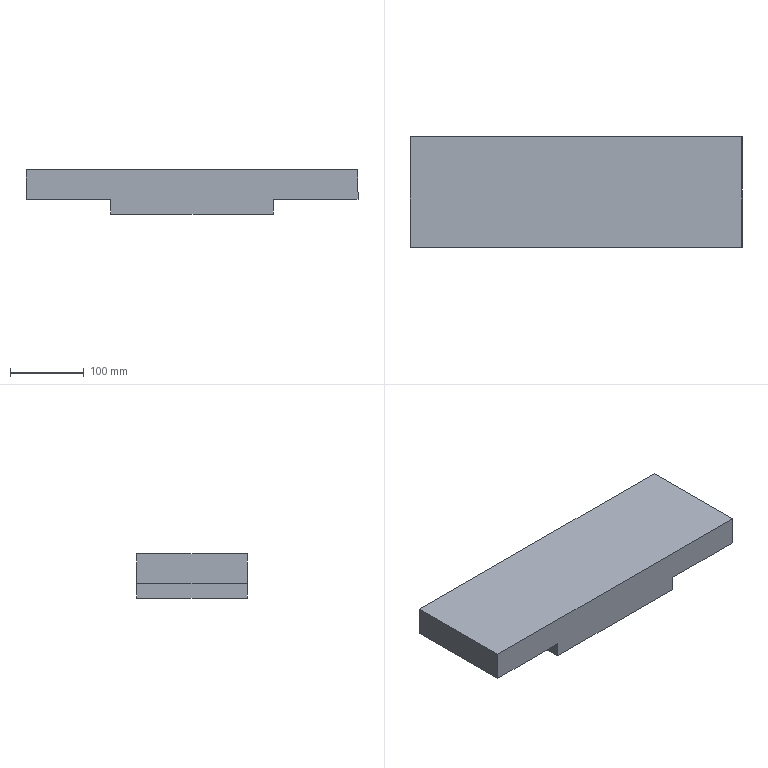Part | SolidWorks | features Extrusion 1 | 1 solid | 10 faces | box 450 x 150 x 60 mm | volume 3360000 mm3 | plane 10
STEP:
#1=CARTESIAN_POINT('',(0.,0.,0.));
#2=VERTEX_POINT('',#1);
#3=CARTESIAN_POINT('',(0.,0.,40.));
#4=VERTEX_POINT('',#3);
#5=CARTESIAN_POINT('',(0.,0.,0.));
#6=DIRECTION('',(0.,0.,1.));
#7=VECTOR('',#6,1000.);
#8=LINE('',#5,#7);
#9=EDGE_CURVE('',#2,#4,#8,.T.);
#10=ORIENTED_EDGE('',*,*,#9,.T.);
#11=CARTESIAN_POINT('',(0.,150.,40.));
#12=VERTEX_POINT('',#11);
#13=CARTESIAN_POINT('',(0.,150.,40.));
#14=DIRECTION('',(0.,-1.,0.));
#15=VECTOR('',#14,1000.);
#16=LINE('',#13,#15);
#17=EDGE_CURVE('',#12,#4,#16,.T.);
#18=ORIENTED_EDGE('',*,*,#17,.F.);
#19=CARTESIAN_POINT('',(0.,150.,0.));
#20=VERTEX_POINT('',#19);
#21=CARTESIAN_POINT('',(0.,150.,0.));
#22=DIRECTION('',(0.,0.,1.));
#23=VECTOR('',#22,1000.);
#24=LINE('',#21,#23);
#25=EDGE_CURVE('',#20,#12,#24,.T.);
#26=ORIENTED_EDGE('',*,*,#25,.F.);
#27=CARTESIAN_POINT('',(0.,150.,0.));
#28=DIRECTION('',(0.,-1.,0.));
#29=VECTOR('',#28,1000.);
#30=LINE('',#27,#29);
#31=EDGE_CURVE('',#20,#2,#30,.T.);
#32=ORIENTED_EDGE('',*,*,#31,.T.);
#33=EDGE_LOOP('',(#10,#18,#26,#32));
#34=FACE_OUTER_BOUND('',#33,.T.);
#35=CARTESIAN_POINT('',(0.,150.,0.));
#36=DIRECTION('',(1.,0.,0.));
#37=DIRECTION('',(0.,0.,-1.));
#38=AXIS2_PLACEMENT_3D('',#35,#36,#37);
#39=PLANE('',#38);
#40=ADVANCED_FACE('',(#34),#39,.F.);
#41=CARTESIAN_POINT('',(450.,0.,40.));
#42=VERTEX_POINT('',#41);
#43=CARTESIAN_POINT('',(0.,0.,40.));
#44=DIRECTION('',(1.,0.,0.));
#45=VECTOR('',#44,1000.);
#46=LINE('',#43,#45);
#47=EDGE_CURVE('',#4,#42,#46,.T.);
#48=ORIENTED_EDGE('',*,*,#47,.T.);
#49=CARTESIAN_POINT('',(450.,150.,40.));
#50=VERTEX_POINT('',#49);
#51=CARTESIAN_POINT('',(450.,150.,40.));
#52=DIRECTION('',(0.,-1.,0.));
#53=VECTOR('',#52,1000.);
#54=LINE('',#51,#53);
#55=EDGE_CURVE('',#50,#42,#54,.T.);
#56=ORIENTED_EDGE('',*,*,#55,.F.);
#57=CARTESIAN_POINT('',(0.,150.,40.));
#58=DIRECTION('',(1.,0.,0.));
#59=VECTOR('',#58,1000.);
#60=LINE('',#57,#59);
#61=EDGE_CURVE('',#12,#50,#60,.T.);
#62=ORIENTED_EDGE('',*,*,#61,.F.);
#63=ORIENTED_EDGE('',*,*,#17,.T.);
#64=EDGE_LOOP('',(#48,#56,#62,#63));
#65=FACE_OUTER_BOUND('',#64,.T.);
#66=CARTESIAN_POINT('',(0.,150.,40.));
#67=DIRECTION('',(0.,0.,-1.));
#68=DIRECTION('',(-1.,0.,0.));
#69=AXIS2_PLACEMENT_3D('',#66,#67,#68);
#70=PLANE('',#69);
#71=ADVANCED_FACE('',(#65),#70,.F.);
#72=CARTESIAN_POINT('',(450.,0.,0.));
#73=VERTEX_POINT('',#72);
#74=CARTESIAN_POINT('',(450.,0.,0.));
#75=DIRECTION('',(0.,0.,-1.));
#76=VECTOR('',#75,1000.);
#77=LINE('',#74,#76);
#78=EDGE_CURVE('',#42,#73,#77,.T.);
#79=ORIENTED_EDGE('',*,*,#78,.T.);
#80=CARTESIAN_POINT('',(450.,150.,0.));
#81=VERTEX_POINT('',#80);
#82=CARTESIAN_POINT('',(450.,150.,0.));
#83=DIRECTION('',(0.,-1.,0.));
#84=VECTOR('',#83,1000.);
#85=LINE('',#82,#84);
#86=EDGE_CURVE('',#81,#73,#85,.T.);
#87=ORIENTED_EDGE('',*,*,#86,.F.);
#88=CARTESIAN_POINT('',(450.,150.,0.));
#89=DIRECTION('',(0.,0.,-1.));
#90=VECTOR('',#89,1000.);
#91=LINE('',#88,#90);
#92=EDGE_CURVE('',#50,#81,#91,.T.);
#93=ORIENTED_EDGE('',*,*,#92,.F.);
#94=ORIENTED_EDGE('',*,*,#55,.T.);
#95=EDGE_LOOP('',(#79,#87,#93,#94));
#96=FACE_OUTER_BOUND('',#95,.T.);
#97=CARTESIAN_POINT('',(450.,150.,0.));
#98=DIRECTION('',(-1.,0.,0.));
#99=DIRECTION('',(0.,0.,1.));
#100=AXIS2_PLACEMENT_3D('',#97,#98,#99);
#101=PLANE('',#100);
#102=ADVANCED_FACE('',(#96),#101,.F.);
#103=CARTESIAN_POINT('',(335.,0.,0.));
#104=VERTEX_POINT('',#103);
#105=CARTESIAN_POINT('',(335.,0.,0.));
#106=DIRECTION('',(-1.,0.,0.));
#107=VECTOR('',#106,1000.);
#108=LINE('',#105,#107);
#109=EDGE_CURVE('',#73,#104,#108,.T.);
#110=ORIENTED_EDGE('',*,*,#109,.T.);
#111=CARTESIAN_POINT('',(335.,150.,0.));
#112=VERTEX_POINT('',#111);
#113=CARTESIAN_POINT('',(335.,150.,0.));
#114=DIRECTION('',(0.,-1.,0.));
#115=VECTOR('',#114,1000.);
#116=LINE('',#113,#115);
#117=EDGE_CURVE('',#112,#104,#116,.T.);
#118=ORIENTED_EDGE('',*,*,#117,.F.);
#119=CARTESIAN_POINT('',(335.,150.,0.));
#120=DIRECTION('',(-1.,0.,0.));
#121=VECTOR('',#120,1000.);
#122=LINE('',#119,#121);
#123=EDGE_CURVE('',#81,#112,#122,.T.);
#124=ORIENTED_EDGE('',*,*,#123,.F.);
#125=ORIENTED_EDGE('',*,*,#86,.T.);
#126=EDGE_LOOP('',(#110,#118,#124,#125));
#127=FACE_OUTER_BOUND('',#126,.T.);
#128=CARTESIAN_POINT('',(335.,150.,0.));
#129=DIRECTION('',(0.,0.,1.));
#130=DIRECTION('',(1.,0.,0.));
#131=AXIS2_PLACEMENT_3D('',#128,#129,#130);
#132=PLANE('',#131);
#133=ADVANCED_FACE('',(#127),#132,.F.);
#134=CARTESIAN_POINT('',(335.,0.,-20.));
#135=VERTEX_POINT('',#134);
#136=CARTESIAN_POINT('',(335.,0.,-20.));
#137=DIRECTION('',(0.,0.,-1.));
#138=VECTOR('',#137,1000.);
#139=LINE('',#136,#138);
#140=EDGE_CURVE('',#104,#135,#139,.T.);
#141=ORIENTED_EDGE('',*,*,#140,.T.);
#142=CARTESIAN_POINT('',(335.,150.,-20.));
#143=VERTEX_POINT('',#142);
#144=CARTESIAN_POINT('',(335.,150.,-20.));
#145=DIRECTION('',(0.,-1.,0.));
#146=VECTOR('',#145,1000.);
#147=LINE('',#144,#146);
#148=EDGE_CURVE('',#143,#135,#147,.T.);
#149=ORIENTED_EDGE('',*,*,#148,.F.);
#150=CARTESIAN_POINT('',(335.,150.,-20.));
#151=DIRECTION('',(0.,0.,-1.));
#152=VECTOR('',#151,1000.);
#153=LINE('',#150,#152);
#154=EDGE_CURVE('',#112,#143,#153,.T.);
#155=ORIENTED_EDGE('',*,*,#154,.F.);
#156=ORIENTED_EDGE('',*,*,#117,.T.);
#157=EDGE_LOOP('',(#141,#149,#155,#156));
#158=FACE_OUTER_BOUND('',#157,.T.);
#159=CARTESIAN_POINT('',(335.,150.,-20.));
#160=DIRECTION('',(-1.,0.,0.));
#161=DIRECTION('',(0.,0.,1.));
#162=AXIS2_PLACEMENT_3D('',#159,#160,#161);
#163=PLANE('',#162);
#164=ADVANCED_FACE('',(#158),#163,.F.);
#165=CARTESIAN_POINT('',(115.,0.,-20.));
#166=VERTEX_POINT('',#165);
#167=CARTESIAN_POINT('',(115.,0.,-20.));
#168=DIRECTION('',(-1.,0.,0.));
#169=VECTOR('',#168,1000.);
#170=LINE('',#167,#169);
#171=EDGE_CURVE('',#135,#166,#170,.T.);
#172=ORIENTED_EDGE('',*,*,#171,.T.);
#173=CARTESIAN_POINT('',(115.,150.,-20.));
#174=VERTEX_POINT('',#173);
#175=CARTESIAN_POINT('',(115.,150.,-20.));
#176=DIRECTION('',(0.,-1.,0.));
#177=VECTOR('',#176,1000.);
#178=LINE('',#175,#177);
#179=EDGE_CURVE('',#174,#166,#178,.T.);
#180=ORIENTED_EDGE('',*,*,#179,.F.);
#181=CARTESIAN_POINT('',(115.,150.,-20.));
#182=DIRECTION('',(-1.,0.,0.));
#183=VECTOR('',#182,1000.);
#184=LINE('',#181,#183);
#185=EDGE_CURVE('',#143,#174,#184,.T.);
#186=ORIENTED_EDGE('',*,*,#185,.F.);
#187=ORIENTED_EDGE('',*,*,#148,.T.);
#188=EDGE_LOOP('',(#172,#180,#186,#187));
#189=FACE_OUTER_BOUND('',#188,.T.);
#190=CARTESIAN_POINT('',(115.,150.,-20.));
#191=DIRECTION('',(0.,0.,1.));
#192=DIRECTION('',(1.,0.,0.));
#193=AXIS2_PLACEMENT_3D('',#190,#191,#192);
#194=PLANE('',#193);
#195=ADVANCED_FACE('',(#189),#194,.F.);
#196=CARTESIAN_POINT('',(115.,0.,0.));
#197=VERTEX_POINT('',#196);
#198=CARTESIAN_POINT('',(115.,0.,0.));
#199=DIRECTION('',(0.,0.,1.));
#200=VECTOR('',#199,1000.);
#201=LINE('',#198,#200);
#202=EDGE_CURVE('',#166,#197,#201,.T.);
#203=ORIENTED_EDGE('',*,*,#202,.T.);
#204=CARTESIAN_POINT('',(115.,150.,0.));
#205=VERTEX_POINT('',#204);
#206=CARTESIAN_POINT('',(115.,150.,0.));
#207=DIRECTION('',(0.,-1.,0.));
#208=VECTOR('',#207,1000.);
#209=LINE('',#206,#208);
#210=EDGE_CURVE('',#205,#197,#209,.T.);
#211=ORIENTED_EDGE('',*,*,#210,.F.);
#212=CARTESIAN_POINT('',(115.,150.,0.));
#213=DIRECTION('',(0.,0.,1.));
#214=VECTOR('',#213,1000.);
#215=LINE('',#212,#214);
#216=EDGE_CURVE('',#174,#205,#215,.T.);
#217=ORIENTED_EDGE('',*,*,#216,.F.);
#218=ORIENTED_EDGE('',*,*,#179,.T.);
#219=EDGE_LOOP('',(#203,#211,#217,#218));
#220=FACE_OUTER_BOUND('',#219,.T.);
#221=CARTESIAN_POINT('',(115.,150.,0.));
#222=DIRECTION('',(1.,0.,0.));
#223=DIRECTION('',(0.,0.,-1.));
#224=AXIS2_PLACEMENT_3D('',#221,#222,#223);
#225=PLANE('',#224);
#226=ADVANCED_FACE('',(#220),#225,.F.);
#227=CARTESIAN_POINT('',(0.,0.,0.));
#228=DIRECTION('',(-1.,0.,0.));
#229=VECTOR('',#228,1000.);
#230=LINE('',#227,#229);
#231=EDGE_CURVE('',#197,#2,#230,.T.);
#232=ORIENTED_EDGE('',*,*,#231,.T.);
#233=ORIENTED_EDGE('',*,*,#31,.F.);
#234=CARTESIAN_POINT('',(0.,150.,0.));
#235=DIRECTION('',(-1.,0.,0.));
#236=VECTOR('',#235,1000.);
#237=LINE('',#234,#236);
#238=EDGE_CURVE('',#205,#20,#237,.T.);
#239=ORIENTED_EDGE('',*,*,#238,.F.);
#240=ORIENTED_EDGE('',*,*,#210,.T.);
#241=EDGE_LOOP('',(#232,#233,#239,#240));
#242=FACE_OUTER_BOUND('',#241,.T.);
#243=CARTESIAN_POINT('',(0.,150.,0.));
#244=DIRECTION('',(0.,0.,1.));
#245=DIRECTION('',(1.,0.,0.));
#246=AXIS2_PLACEMENT_3D('',#243,#244,#245);
#247=PLANE('',#246);
#248=ADVANCED_FACE('',(#242),#247,.F.);
#249=ORIENTED_EDGE('',*,*,#25,.T.);
#250=ORIENTED_EDGE('',*,*,#61,.T.);
#251=ORIENTED_EDGE('',*,*,#92,.T.);
#252=ORIENTED_EDGE('',*,*,#123,.T.);
#253=ORIENTED_EDGE('',*,*,#154,.T.);
#254=ORIENTED_EDGE('',*,*,#185,.T.);
#255=ORIENTED_EDGE('',*,*,#216,.T.);
#256=ORIENTED_EDGE('',*,*,#238,.T.);
#257=EDGE_LOOP('',(#249,#250,#251,#252,#253,#254,#255,#256));
#258=FACE_OUTER_BOUND('',#257,.T.);
#259=CARTESIAN_POINT('',(0.,150.,0.));
#260=DIRECTION('',(0.,1.,0.));
#261=DIRECTION('',(0.,0.,1.));
#262=AXIS2_PLACEMENT_3D('',#259,#260,#261);
#263=PLANE('',#262);
#264=ADVANCED_FACE('',(#258),#263,.T.);
#265=ORIENTED_EDGE('',*,*,#9,.F.);
#266=ORIENTED_EDGE('',*,*,#231,.F.);
#267=ORIENTED_EDGE('',*,*,#202,.F.);
#268=ORIENTED_EDGE('',*,*,#171,.F.);
#269=ORIENTED_EDGE('',*,*,#140,.F.);
#270=ORIENTED_EDGE('',*,*,#109,.F.);
#271=ORIENTED_EDGE('',*,*,#78,.F.);
#272=ORIENTED_EDGE('',*,*,#47,.F.);
#273=EDGE_LOOP('',(#265,#266,#267,#268,#269,#270,#271,#272));
#274=FACE_OUTER_BOUND('',#273,.T.);
#275=CARTESIAN_POINT('',(0.,0.,0.));
#276=DIRECTION('',(0.,1.,0.));
#277=DIRECTION('',(0.,0.,1.));
#278=AXIS2_PLACEMENT_3D('',#275,#276,#277);
#279=PLANE('',#278);
#280=ADVANCED_FACE('',(#274),#279,.F.);
#281=CLOSED_SHELL('',(#40,#71,#102,#133,#164,#195,#226,#248,#264,#280));
#282=MANIFOLD_SOLID_BREP('',#281);
#283=CARTESIAN_POINT('',(0.,0.,0.));
#284=DIRECTION('',(0.,0.,1.));
#285=DIRECTION('',(1.,0.,0.));
#286=AXIS2_PLACEMENT_3D('',#283,#284,#285);
#287=(LENGTH_UNIT()NAMED_UNIT(*)SI_UNIT(.MILLI.,.METRE.));
#288=UNCERTAINTY_MEASURE_WITH_UNIT(LENGTH_MEASURE(0.00001),#287,'','');
#289=(NAMED_UNIT(*)PLANE_ANGLE_UNIT()SI_UNIT($,.RADIAN.));
#290=(NAMED_UNIT(*)SI_UNIT($,.STERADIAN.)SOLID_ANGLE_UNIT());
#291=(GEOMETRIC_REPRESENTATION_CONTEXT(3)GLOBAL_UNCERTAINTY_ASSIGNED_CONTEXT((#288))GLOBAL_UNIT_ASSIGNED_CONTEXT((#287,#289,#290))REPRESENTATION_CONTEXT('',''));
#292=ADVANCED_BREP_SHAPE_REPRESENTATION('',(#282,#286),#291);